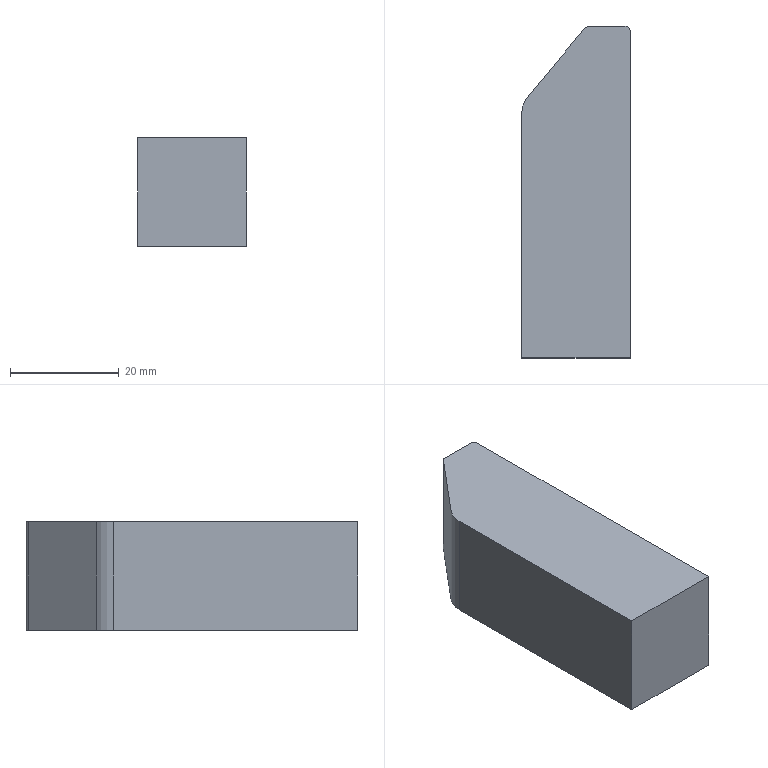Part | STEP file | lll_id934_x_t | 1 solid | 10 faces | box 20 x 61.082 x 20 mm | volume 22704 mm3 | plane 7 | cylinder 3 | commonest cylinder face diameters 2 x2 10 x1
STEP:
#1=CARTESIAN_POINT('',(775.37,-399.832,2.5));
#2=VERTEX_POINT('',#1);
#3=CARTESIAN_POINT('',(775.37,-354.871,2.5));
#4=VERTEX_POINT('',#3);
#5=CARTESIAN_POINT('',(775.37,-399.832,2.5));
#6=DIRECTION('',(0.,1.,0.));
#7=VECTOR('',#6,1.);
#8=LINE('',#5,#7);
#9=EDGE_CURVE('',#2,#4,#8,.T.);
#10=ORIENTED_EDGE('',*,*,#9,.T.);
#11=CARTESIAN_POINT('',(775.37,-354.871,-17.5));
#12=VERTEX_POINT('',#11);
#13=CARTESIAN_POINT('',(775.37,-354.871,-17.5));
#14=DIRECTION('',(0.,0.,1.));
#15=VECTOR('',#14,1.);
#16=LINE('',#13,#15);
#17=EDGE_CURVE('',#12,#4,#16,.T.);
#18=ORIENTED_EDGE('',*,*,#17,.F.);
#19=CARTESIAN_POINT('',(775.37,-399.832,-17.5));
#20=VERTEX_POINT('',#19);
#21=CARTESIAN_POINT('',(775.37,-399.832,-17.5));
#22=DIRECTION('',(0.,1.,0.));
#23=VECTOR('',#22,1.);
#24=LINE('',#21,#23);
#25=EDGE_CURVE('',#20,#12,#24,.T.);
#26=ORIENTED_EDGE('',*,*,#25,.F.);
#27=CARTESIAN_POINT('',(775.37,-399.832,-17.5));
#28=DIRECTION('',(0.,0.,1.));
#29=VECTOR('',#28,1.);
#30=LINE('',#27,#29);
#31=EDGE_CURVE('',#20,#2,#30,.T.);
#32=ORIENTED_EDGE('',*,*,#31,.T.);
#33=EDGE_LOOP('',(#10,#18,#26,#32));
#34=FACE_OUTER_BOUND('',#33,.T.);
#35=CARTESIAN_POINT('',(775.37,-399.832,-17.5));
#36=DIRECTION('',(-1.,0.,0.));
#37=DIRECTION('',(0.,0.,1.));
#38=AXIS2_PLACEMENT_3D('',#35,#36,#37);
#39=PLANE('',#38);
#40=ADVANCED_FACE('',(#34),#39,.T.);
#41=CARTESIAN_POINT('',(776.54,-351.657,2.5));
#42=VERTEX_POINT('',#41);
#43=CARTESIAN_POINT('',(780.37,-354.871,2.5));
#44=DIRECTION('',(0.,0.,-1.));
#45=DIRECTION('',(-1.,0.,0.));
#46=AXIS2_PLACEMENT_3D('',#43,#44,#45);
#47=CIRCLE('',#46,5.);
#48=EDGE_CURVE('',#4,#42,#47,.T.);
#49=ORIENTED_EDGE('',*,*,#48,.T.);
#50=CARTESIAN_POINT('',(776.54,-351.657,-17.5));
#51=VERTEX_POINT('',#50);
#52=CARTESIAN_POINT('',(776.54,-351.657,-17.5));
#53=DIRECTION('',(0.,0.,1.));
#54=VECTOR('',#53,1.);
#55=LINE('',#52,#54);
#56=EDGE_CURVE('',#51,#42,#55,.T.);
#57=ORIENTED_EDGE('',*,*,#56,.F.);
#58=CARTESIAN_POINT('',(780.37,-354.871,-17.5));
#59=DIRECTION('',(0.,0.,-1.));
#60=DIRECTION('',(-1.,0.,0.));
#61=AXIS2_PLACEMENT_3D('',#58,#59,#60);
#62=CIRCLE('',#61,5.);
#63=EDGE_CURVE('',#12,#51,#62,.T.);
#64=ORIENTED_EDGE('',*,*,#63,.F.);
#65=ORIENTED_EDGE('',*,*,#17,.T.);
#66=EDGE_LOOP('',(#49,#57,#64,#65));
#67=FACE_OUTER_BOUND('',#66,.T.);
#68=CARTESIAN_POINT('',(780.37,-354.871,-17.5));
#69=DIRECTION('',(0.,0.,1.));
#70=DIRECTION('',(1.,0.,0.));
#71=AXIS2_PLACEMENT_3D('',#68,#69,#70);
#72=CYLINDRICAL_SURFACE('',#71,5.);
#73=ADVANCED_FACE('',(#67),#72,.T.);
#74=CARTESIAN_POINT('',(787.071,-339.107,2.5));
#75=VERTEX_POINT('',#74);
#76=CARTESIAN_POINT('',(776.54,-351.657,2.5));
#77=DIRECTION('',(0.6428,0.766,0.));
#78=VECTOR('',#77,1.);
#79=LINE('',#76,#78);
#80=EDGE_CURVE('',#42,#75,#79,.T.);
#81=ORIENTED_EDGE('',*,*,#80,.T.);
#82=CARTESIAN_POINT('',(787.071,-339.107,-17.5));
#83=VERTEX_POINT('',#82);
#84=CARTESIAN_POINT('',(787.071,-339.107,-17.5));
#85=DIRECTION('',(0.,0.,1.));
#86=VECTOR('',#85,1.);
#87=LINE('',#84,#86);
#88=EDGE_CURVE('',#83,#75,#87,.T.);
#89=ORIENTED_EDGE('',*,*,#88,.F.);
#90=CARTESIAN_POINT('',(776.54,-351.657,-17.5));
#91=DIRECTION('',(0.6428,0.766,0.));
#92=VECTOR('',#91,1.);
#93=LINE('',#90,#92);
#94=EDGE_CURVE('',#51,#83,#93,.T.);
#95=ORIENTED_EDGE('',*,*,#94,.F.);
#96=ORIENTED_EDGE('',*,*,#56,.T.);
#97=EDGE_LOOP('',(#81,#89,#95,#96));
#98=FACE_OUTER_BOUND('',#97,.T.);
#99=CARTESIAN_POINT('',(776.54,-351.657,-17.5));
#100=DIRECTION('',(-0.766,0.6428,0.));
#101=DIRECTION('',(-0.6428,-0.766,0.));
#102=AXIS2_PLACEMENT_3D('',#99,#100,#101);
#103=PLANE('',#102);
#104=ADVANCED_FACE('',(#98),#103,.T.);
#105=CARTESIAN_POINT('',(787.837,-338.75,2.5));
#106=VERTEX_POINT('',#105);
#107=CARTESIAN_POINT('',(787.837,-339.75,2.5));
#108=DIRECTION('',(0.,0.,-1.));
#109=DIRECTION('',(-1.,0.,0.));
#110=AXIS2_PLACEMENT_3D('',#107,#108,#109);
#111=CIRCLE('',#110,1.);
#112=EDGE_CURVE('',#75,#106,#111,.T.);
#113=ORIENTED_EDGE('',*,*,#112,.T.);
#114=CARTESIAN_POINT('',(787.837,-338.75,-17.5));
#115=VERTEX_POINT('',#114);
#116=CARTESIAN_POINT('',(787.837,-338.75,-17.5));
#117=DIRECTION('',(0.,0.,1.));
#118=VECTOR('',#117,1.);
#119=LINE('',#116,#118);
#120=EDGE_CURVE('',#115,#106,#119,.T.);
#121=ORIENTED_EDGE('',*,*,#120,.F.);
#122=CARTESIAN_POINT('',(787.837,-339.75,-17.5));
#123=DIRECTION('',(0.,0.,-1.));
#124=DIRECTION('',(-1.,0.,0.));
#125=AXIS2_PLACEMENT_3D('',#122,#123,#124);
#126=CIRCLE('',#125,1.);
#127=EDGE_CURVE('',#83,#115,#126,.T.);
#128=ORIENTED_EDGE('',*,*,#127,.F.);
#129=ORIENTED_EDGE('',*,*,#88,.T.);
#130=EDGE_LOOP('',(#113,#121,#128,#129));
#131=FACE_OUTER_BOUND('',#130,.T.);
#132=CARTESIAN_POINT('',(787.837,-339.75,-17.5));
#133=DIRECTION('',(0.,0.,1.));
#134=DIRECTION('',(1.,0.,0.));
#135=AXIS2_PLACEMENT_3D('',#132,#133,#134);
#136=CYLINDRICAL_SURFACE('',#135,1.);
#137=ADVANCED_FACE('',(#131),#136,.T.);
#138=CARTESIAN_POINT('',(794.37,-338.75,2.5));
#139=VERTEX_POINT('',#138);
#140=CARTESIAN_POINT('',(787.837,-338.75,2.5));
#141=DIRECTION('',(1.,0.,0.));
#142=VECTOR('',#141,1.);
#143=LINE('',#140,#142);
#144=EDGE_CURVE('',#106,#139,#143,.T.);
#145=ORIENTED_EDGE('',*,*,#144,.T.);
#146=CARTESIAN_POINT('',(794.37,-338.75,-17.5));
#147=VERTEX_POINT('',#146);
#148=CARTESIAN_POINT('',(794.37,-338.75,-17.5));
#149=DIRECTION('',(0.,0.,1.));
#150=VECTOR('',#149,1.);
#151=LINE('',#148,#150);
#152=EDGE_CURVE('',#147,#139,#151,.T.);
#153=ORIENTED_EDGE('',*,*,#152,.F.);
#154=CARTESIAN_POINT('',(787.837,-338.75,-17.5));
#155=DIRECTION('',(1.,0.,0.));
#156=VECTOR('',#155,1.);
#157=LINE('',#154,#156);
#158=EDGE_CURVE('',#115,#147,#157,.T.);
#159=ORIENTED_EDGE('',*,*,#158,.F.);
#160=ORIENTED_EDGE('',*,*,#120,.T.);
#161=EDGE_LOOP('',(#145,#153,#159,#160));
#162=FACE_OUTER_BOUND('',#161,.T.);
#163=CARTESIAN_POINT('',(787.837,-338.75,-17.5));
#164=DIRECTION('',(0.,1.,0.));
#165=DIRECTION('',(-1.,0.,0.));
#166=AXIS2_PLACEMENT_3D('',#163,#164,#165);
#167=PLANE('',#166);
#168=ADVANCED_FACE('',(#162),#167,.T.);
#169=CARTESIAN_POINT('',(795.37,-339.75,2.5));
#170=VERTEX_POINT('',#169);
#171=CARTESIAN_POINT('',(794.37,-339.75,2.5));
#172=DIRECTION('',(0.,0.,-1.));
#173=DIRECTION('',(-1.,0.,0.));
#174=AXIS2_PLACEMENT_3D('',#171,#172,#173);
#175=CIRCLE('',#174,1.);
#176=EDGE_CURVE('',#139,#170,#175,.T.);
#177=ORIENTED_EDGE('',*,*,#176,.T.);
#178=CARTESIAN_POINT('',(795.37,-339.75,-17.5));
#179=VERTEX_POINT('',#178);
#180=CARTESIAN_POINT('',(795.37,-339.75,-17.5));
#181=DIRECTION('',(0.,0.,1.));
#182=VECTOR('',#181,1.);
#183=LINE('',#180,#182);
#184=EDGE_CURVE('',#179,#170,#183,.T.);
#185=ORIENTED_EDGE('',*,*,#184,.F.);
#186=CARTESIAN_POINT('',(794.37,-339.75,-17.5));
#187=DIRECTION('',(0.,0.,-1.));
#188=DIRECTION('',(-1.,0.,0.));
#189=AXIS2_PLACEMENT_3D('',#186,#187,#188);
#190=CIRCLE('',#189,1.);
#191=EDGE_CURVE('',#147,#179,#190,.T.);
#192=ORIENTED_EDGE('',*,*,#191,.F.);
#193=ORIENTED_EDGE('',*,*,#152,.T.);
#194=EDGE_LOOP('',(#177,#185,#192,#193));
#195=FACE_OUTER_BOUND('',#194,.T.);
#196=CARTESIAN_POINT('',(794.37,-339.75,-17.5));
#197=DIRECTION('',(0.,0.,1.));
#198=DIRECTION('',(1.,0.,0.));
#199=AXIS2_PLACEMENT_3D('',#196,#197,#198);
#200=CYLINDRICAL_SURFACE('',#199,1.);
#201=ADVANCED_FACE('',(#195),#200,.T.);
#202=CARTESIAN_POINT('',(795.37,-399.832,2.5));
#203=VERTEX_POINT('',#202);
#204=CARTESIAN_POINT('',(795.37,-339.75,2.5));
#205=DIRECTION('',(0.,-1.,0.));
#206=VECTOR('',#205,1.);
#207=LINE('',#204,#206);
#208=EDGE_CURVE('',#170,#203,#207,.T.);
#209=ORIENTED_EDGE('',*,*,#208,.T.);
#210=CARTESIAN_POINT('',(795.37,-399.832,-17.5));
#211=VERTEX_POINT('',#210);
#212=CARTESIAN_POINT('',(795.37,-399.832,-17.5));
#213=DIRECTION('',(0.,0.,1.));
#214=VECTOR('',#213,1.);
#215=LINE('',#212,#214);
#216=EDGE_CURVE('',#211,#203,#215,.T.);
#217=ORIENTED_EDGE('',*,*,#216,.F.);
#218=CARTESIAN_POINT('',(795.37,-339.75,-17.5));
#219=DIRECTION('',(0.,-1.,0.));
#220=VECTOR('',#219,1.);
#221=LINE('',#218,#220);
#222=EDGE_CURVE('',#179,#211,#221,.T.);
#223=ORIENTED_EDGE('',*,*,#222,.F.);
#224=ORIENTED_EDGE('',*,*,#184,.T.);
#225=EDGE_LOOP('',(#209,#217,#223,#224));
#226=FACE_OUTER_BOUND('',#225,.T.);
#227=CARTESIAN_POINT('',(795.37,-339.75,-17.5));
#228=DIRECTION('',(1.,0.,0.));
#229=DIRECTION('',(0.,0.,-1.));
#230=AXIS2_PLACEMENT_3D('',#227,#228,#229);
#231=PLANE('',#230);
#232=ADVANCED_FACE('',(#226),#231,.T.);
#233=CARTESIAN_POINT('',(795.37,-399.832,2.5));
#234=DIRECTION('',(-1.,0.,0.));
#235=VECTOR('',#234,1.);
#236=LINE('',#233,#235);
#237=EDGE_CURVE('',#203,#2,#236,.T.);
#238=ORIENTED_EDGE('',*,*,#237,.T.);
#239=ORIENTED_EDGE('',*,*,#31,.F.);
#240=CARTESIAN_POINT('',(795.37,-399.832,-17.5));
#241=DIRECTION('',(-1.,0.,0.));
#242=VECTOR('',#241,1.);
#243=LINE('',#240,#242);
#244=EDGE_CURVE('',#211,#20,#243,.T.);
#245=ORIENTED_EDGE('',*,*,#244,.F.);
#246=ORIENTED_EDGE('',*,*,#216,.T.);
#247=EDGE_LOOP('',(#238,#239,#245,#246));
#248=FACE_OUTER_BOUND('',#247,.T.);
#249=CARTESIAN_POINT('',(795.37,-399.832,-17.5));
#250=DIRECTION('',(0.,-1.,0.));
#251=DIRECTION('',(0.,0.,1.));
#252=AXIS2_PLACEMENT_3D('',#249,#250,#251);
#253=PLANE('',#252);
#254=ADVANCED_FACE('',(#248),#253,.T.);
#255=ORIENTED_EDGE('',*,*,#25,.T.);
#256=ORIENTED_EDGE('',*,*,#63,.T.);
#257=ORIENTED_EDGE('',*,*,#94,.T.);
#258=ORIENTED_EDGE('',*,*,#127,.T.);
#259=ORIENTED_EDGE('',*,*,#158,.T.);
#260=ORIENTED_EDGE('',*,*,#191,.T.);
#261=ORIENTED_EDGE('',*,*,#222,.T.);
#262=ORIENTED_EDGE('',*,*,#244,.T.);
#263=EDGE_LOOP('',(#255,#256,#257,#258,#259,#260,#261,#262));
#264=FACE_OUTER_BOUND('',#263,.T.);
#265=CARTESIAN_POINT('',(780.37,-354.871,-17.5));
#266=DIRECTION('',(0.,0.,1.));
#267=DIRECTION('',(1.,0.,0.));
#268=AXIS2_PLACEMENT_3D('',#265,#266,#267);
#269=PLANE('',#268);
#270=ADVANCED_FACE('',(#264),#269,.F.);
#271=ORIENTED_EDGE('',*,*,#9,.F.);
#272=ORIENTED_EDGE('',*,*,#237,.F.);
#273=ORIENTED_EDGE('',*,*,#208,.F.);
#274=ORIENTED_EDGE('',*,*,#176,.F.);
#275=ORIENTED_EDGE('',*,*,#144,.F.);
#276=ORIENTED_EDGE('',*,*,#112,.F.);
#277=ORIENTED_EDGE('',*,*,#80,.F.);
#278=ORIENTED_EDGE('',*,*,#48,.F.);
#279=EDGE_LOOP('',(#271,#272,#273,#274,#275,#276,#277,#278));
#280=FACE_OUTER_BOUND('',#279,.T.);
#281=CARTESIAN_POINT('',(780.37,-354.871,2.5));
#282=DIRECTION('',(0.,0.,1.));
#283=DIRECTION('',(1.,0.,0.));
#284=AXIS2_PLACEMENT_3D('',#281,#282,#283);
#285=PLANE('',#284);
#286=ADVANCED_FACE('',(#280),#285,.T.);
#287=CLOSED_SHELL('',(#40,#73,#104,#137,#168,#201,#232,#254,#270,#286));
#288=MANIFOLD_SOLID_BREP('',#287);
#289=(LENGTH_UNIT()NAMED_UNIT(*)SI_UNIT(.MILLI.,.METRE.));
#290=UNCERTAINTY_MEASURE_WITH_UNIT(LENGTH_MEASURE(0.00002),#289,'','');
#291=(NAMED_UNIT(*)PLANE_ANGLE_UNIT()SI_UNIT($,.RADIAN.));
#292=PLANE_ANGLE_MEASURE_WITH_UNIT(PLANE_ANGLE_MEASURE(0.01745),#291);
#293=DIMENSIONAL_EXPONENTS(0.,0.,0.,0.,0.,0.,0.);
#294=(CONVERSION_BASED_UNIT('DEGREE',#292)NAMED_UNIT(#293)PLANE_ANGLE_UNIT());
#295=(NAMED_UNIT(*)SI_UNIT($,.STERADIAN.)SOLID_ANGLE_UNIT());
#296=(GEOMETRIC_REPRESENTATION_CONTEXT(3)GLOBAL_UNCERTAINTY_ASSIGNED_CONTEXT((#290))GLOBAL_UNIT_ASSIGNED_CONTEXT((#289,#294,#295))REPRESENTATION_CONTEXT('',''));
#297=ADVANCED_BREP_SHAPE_REPRESENTATION('',(#288),#296);